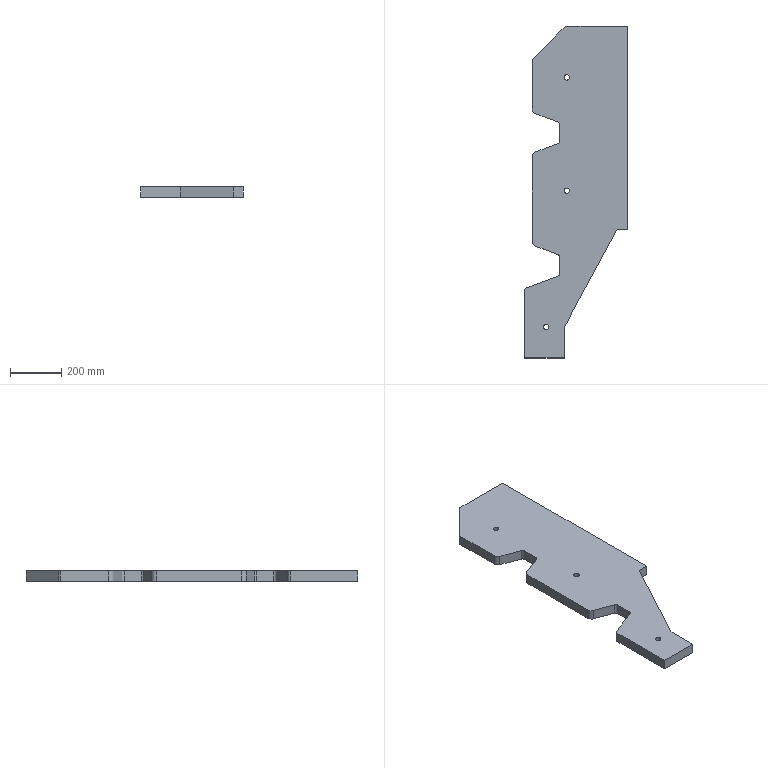Part | SolidWorks | features Fillet 3, ICE 2, 3DProfileFeature 1, Chamfer 1, Extrusion 1, HoleWzd 1 | 1 solid | 34 faces | box 399 x 1290 x 40 mm | volume 14647498 mm3 | plane 18 | cylinder 16 | commonest cylinder face diameters 20 x7 21 x6 40 x3
STEP:
#1=CARTESIAN_POINT('',(174.5,1090.,40.));
#2=VERTEX_POINT('',#1);
#3=CARTESIAN_POINT('',(153.5,1090.,40.));
#4=VERTEX_POINT('',#3);
#5=CARTESIAN_POINT('',(164.,1090.,40.));
#6=DIRECTION('',(0.,0.,-1.));
#7=DIRECTION('',(-1.,0.,0.));
#8=AXIS2_PLACEMENT_3D('',#5,#6,#7);
#9=CIRCLE('',#8,10.5);
#10=EDGE_CURVE('',#2,#4,#9,.T.);
#11=ORIENTED_EDGE('',*,*,#10,.F.);
#12=CARTESIAN_POINT('',(174.5,1090.,0.));
#13=VERTEX_POINT('',#12);
#14=CARTESIAN_POINT('',(174.5,1090.,0.));
#15=DIRECTION('',(0.,0.,-1.));
#16=VECTOR('',#15,1000.);
#17=LINE('',#14,#16);
#18=EDGE_CURVE('',#2,#13,#17,.T.);
#19=ORIENTED_EDGE('',*,*,#18,.T.);
#20=CARTESIAN_POINT('',(153.5,1090.,0.));
#21=VERTEX_POINT('',#20);
#22=CARTESIAN_POINT('',(164.,1090.,0.));
#23=DIRECTION('',(0.,0.,-1.));
#24=DIRECTION('',(-1.,0.,0.));
#25=AXIS2_PLACEMENT_3D('',#22,#23,#24);
#26=CIRCLE('',#25,10.5);
#27=EDGE_CURVE('',#13,#21,#26,.T.);
#28=ORIENTED_EDGE('',*,*,#27,.T.);
#29=CARTESIAN_POINT('',(153.5,1090.,0.));
#30=DIRECTION('',(0.,0.,-1.));
#31=VECTOR('',#30,1000.);
#32=LINE('',#29,#31);
#33=EDGE_CURVE('',#4,#21,#32,.T.);
#34=ORIENTED_EDGE('',*,*,#33,.F.);
#35=EDGE_LOOP('',(#11,#19,#28,#34));
#36=FACE_OUTER_BOUND('',#35,.T.);
#37=CARTESIAN_POINT('',(164.,1090.,0.));
#38=DIRECTION('',(0.,0.,-1.));
#39=DIRECTION('',(-1.,0.,0.));
#40=AXIS2_PLACEMENT_3D('',#37,#38,#39);
#41=CYLINDRICAL_SURFACE('',#40,10.5);
#42=ADVANCED_FACE('',(#36),#41,.F.);
#43=CARTESIAN_POINT('',(174.5,650.,40.));
#44=VERTEX_POINT('',#43);
#45=CARTESIAN_POINT('',(153.5,650.,40.));
#46=VERTEX_POINT('',#45);
#47=CARTESIAN_POINT('',(164.,650.,40.));
#48=DIRECTION('',(0.,0.,-1.));
#49=DIRECTION('',(-1.,0.,0.));
#50=AXIS2_PLACEMENT_3D('',#47,#48,#49);
#51=CIRCLE('',#50,10.5);
#52=EDGE_CURVE('',#44,#46,#51,.T.);
#53=ORIENTED_EDGE('',*,*,#52,.F.);
#54=CARTESIAN_POINT('',(174.5,650.,0.));
#55=VERTEX_POINT('',#54);
#56=CARTESIAN_POINT('',(174.5,650.,0.));
#57=DIRECTION('',(0.,0.,-1.));
#58=VECTOR('',#57,1000.);
#59=LINE('',#56,#58);
#60=EDGE_CURVE('',#44,#55,#59,.T.);
#61=ORIENTED_EDGE('',*,*,#60,.T.);
#62=CARTESIAN_POINT('',(153.5,650.,0.));
#63=VERTEX_POINT('',#62);
#64=CARTESIAN_POINT('',(164.,650.,0.));
#65=DIRECTION('',(0.,0.,-1.));
#66=DIRECTION('',(-1.,0.,0.));
#67=AXIS2_PLACEMENT_3D('',#64,#65,#66);
#68=CIRCLE('',#67,10.5);
#69=EDGE_CURVE('',#55,#63,#68,.T.);
#70=ORIENTED_EDGE('',*,*,#69,.T.);
#71=CARTESIAN_POINT('',(153.5,650.,0.));
#72=DIRECTION('',(0.,0.,-1.));
#73=VECTOR('',#72,1000.);
#74=LINE('',#71,#73);
#75=EDGE_CURVE('',#46,#63,#74,.T.);
#76=ORIENTED_EDGE('',*,*,#75,.F.);
#77=EDGE_LOOP('',(#53,#61,#70,#76));
#78=FACE_OUTER_BOUND('',#77,.T.);
#79=CARTESIAN_POINT('',(164.,650.,0.));
#80=DIRECTION('',(0.,0.,-1.));
#81=DIRECTION('',(-1.,0.,0.));
#82=AXIS2_PLACEMENT_3D('',#79,#80,#81);
#83=CYLINDRICAL_SURFACE('',#82,10.5);
#84=ADVANCED_FACE('',(#78),#83,.F.);
#85=CARTESIAN_POINT('',(94.5,120.,40.));
#86=VERTEX_POINT('',#85);
#87=CARTESIAN_POINT('',(73.5,120.,40.));
#88=VERTEX_POINT('',#87);
#89=CARTESIAN_POINT('',(84.,120.,40.));
#90=DIRECTION('',(0.,0.,-1.));
#91=DIRECTION('',(-1.,0.,0.));
#92=AXIS2_PLACEMENT_3D('',#89,#90,#91);
#93=CIRCLE('',#92,10.5);
#94=EDGE_CURVE('',#86,#88,#93,.T.);
#95=ORIENTED_EDGE('',*,*,#94,.F.);
#96=CARTESIAN_POINT('',(94.5,120.,0.));
#97=VERTEX_POINT('',#96);
#98=CARTESIAN_POINT('',(94.5,120.,0.));
#99=DIRECTION('',(0.,0.,-1.));
#100=VECTOR('',#99,1000.);
#101=LINE('',#98,#100);
#102=EDGE_CURVE('',#86,#97,#101,.T.);
#103=ORIENTED_EDGE('',*,*,#102,.T.);
#104=CARTESIAN_POINT('',(73.5,120.,0.));
#105=VERTEX_POINT('',#104);
#106=CARTESIAN_POINT('',(84.,120.,0.));
#107=DIRECTION('',(0.,0.,-1.));
#108=DIRECTION('',(-1.,0.,0.));
#109=AXIS2_PLACEMENT_3D('',#106,#107,#108);
#110=CIRCLE('',#109,10.5);
#111=EDGE_CURVE('',#97,#105,#110,.T.);
#112=ORIENTED_EDGE('',*,*,#111,.T.);
#113=CARTESIAN_POINT('',(73.5,120.,0.));
#114=DIRECTION('',(0.,0.,-1.));
#115=VECTOR('',#114,1000.);
#116=LINE('',#113,#115);
#117=EDGE_CURVE('',#88,#105,#116,.T.);
#118=ORIENTED_EDGE('',*,*,#117,.F.);
#119=EDGE_LOOP('',(#95,#103,#112,#118));
#120=FACE_OUTER_BOUND('',#119,.T.);
#121=CARTESIAN_POINT('',(84.,120.,0.));
#122=DIRECTION('',(0.,0.,-1.));
#123=DIRECTION('',(-1.,0.,0.));
#124=AXIS2_PLACEMENT_3D('',#121,#122,#123);
#125=CYLINDRICAL_SURFACE('',#124,10.5);
#126=ADVANCED_FACE('',(#120),#125,.F.);
#127=CARTESIAN_POINT('',(0.,263.04,40.));
#128=VERTEX_POINT('',#127);
#129=CARTESIAN_POINT('',(0.,0.,40.));
#130=VERTEX_POINT('',#129);
#131=CARTESIAN_POINT('',(0.,0.,40.));
#132=DIRECTION('',(0.,-1.,0.));
#133=VECTOR('',#132,1000.);
#134=LINE('',#131,#133);
#135=EDGE_CURVE('',#128,#130,#134,.T.);
#136=ORIENTED_EDGE('',*,*,#135,.F.);
#137=CARTESIAN_POINT('',(0.,263.04,0.));
#138=VERTEX_POINT('',#137);
#139=CARTESIAN_POINT('',(0.,263.04,40.));
#140=DIRECTION('',(0.,0.,-1.));
#141=VECTOR('',#140,1000.);
#142=LINE('',#139,#141);
#143=EDGE_CURVE('',#128,#138,#142,.T.);
#144=ORIENTED_EDGE('',*,*,#143,.T.);
#145=CARTESIAN_POINT('',(0.,0.,0.));
#146=VERTEX_POINT('',#145);
#147=CARTESIAN_POINT('',(0.,0.,0.));
#148=DIRECTION('',(0.,-1.,0.));
#149=VECTOR('',#148,1000.);
#150=LINE('',#147,#149);
#151=EDGE_CURVE('',#138,#146,#150,.T.);
#152=ORIENTED_EDGE('',*,*,#151,.T.);
#153=CARTESIAN_POINT('',(0.,0.,40.));
#154=DIRECTION('',(0.,0.,-1.));
#155=VECTOR('',#154,1000.);
#156=LINE('',#153,#155);
#157=EDGE_CURVE('',#130,#146,#156,.T.);
#158=ORIENTED_EDGE('',*,*,#157,.F.);
#159=EDGE_LOOP('',(#136,#144,#152,#158));
#160=FACE_OUTER_BOUND('',#159,.T.);
#161=CARTESIAN_POINT('',(0.,0.,40.));
#162=DIRECTION('',(1.,0.,0.));
#163=DIRECTION('',(0.,0.,-1.));
#164=AXIS2_PLACEMENT_3D('',#161,#162,#163);
#165=PLANE('',#164);
#166=ADVANCED_FACE('',(#160),#165,.F.);
#167=CARTESIAN_POINT('',(154.,0.,0.));
#168=VERTEX_POINT('',#167);
#169=CARTESIAN_POINT('',(0.,0.,0.));
#170=DIRECTION('',(1.,0.,0.));
#171=VECTOR('',#170,1000.);
#172=LINE('',#169,#171);
#173=EDGE_CURVE('',#146,#168,#172,.T.);
#174=ORIENTED_EDGE('',*,*,#173,.T.);
#175=CARTESIAN_POINT('',(154.,0.,40.));
#176=VERTEX_POINT('',#175);
#177=CARTESIAN_POINT('',(154.,0.,40.));
#178=DIRECTION('',(0.,0.,-1.));
#179=VECTOR('',#178,1000.);
#180=LINE('',#177,#179);
#181=EDGE_CURVE('',#176,#168,#180,.T.);
#182=ORIENTED_EDGE('',*,*,#181,.F.);
#183=CARTESIAN_POINT('',(0.,0.,40.));
#184=DIRECTION('',(1.,0.,0.));
#185=VECTOR('',#184,1000.);
#186=LINE('',#183,#185);
#187=EDGE_CURVE('',#130,#176,#186,.T.);
#188=ORIENTED_EDGE('',*,*,#187,.F.);
#189=ORIENTED_EDGE('',*,*,#157,.T.);
#190=EDGE_LOOP('',(#174,#182,#188,#189));
#191=FACE_OUTER_BOUND('',#190,.T.);
#192=CARTESIAN_POINT('',(0.,0.,40.));
#193=DIRECTION('',(0.,1.,0.));
#194=DIRECTION('',(0.,0.,1.));
#195=AXIS2_PLACEMENT_3D('',#192,#193,#194);
#196=PLANE('',#195);
#197=ADVANCED_FACE('',(#191),#196,.F.);
#198=CARTESIAN_POINT('',(154.,120.,0.));
#199=VERTEX_POINT('',#198);
#200=CARTESIAN_POINT('',(154.,0.,0.));
#201=DIRECTION('',(0.,1.,0.));
#202=VECTOR('',#201,1000.);
#203=LINE('',#200,#202);
#204=EDGE_CURVE('',#168,#199,#203,.T.);
#205=ORIENTED_EDGE('',*,*,#204,.T.);
#206=CARTESIAN_POINT('',(154.,120.,40.));
#207=VERTEX_POINT('',#206);
#208=CARTESIAN_POINT('',(154.,120.,40.));
#209=DIRECTION('',(0.,0.,-1.));
#210=VECTOR('',#209,1000.);
#211=LINE('',#208,#210);
#212=EDGE_CURVE('',#207,#199,#211,.T.);
#213=ORIENTED_EDGE('',*,*,#212,.F.);
#214=CARTESIAN_POINT('',(154.,0.,40.));
#215=DIRECTION('',(0.,1.,0.));
#216=VECTOR('',#215,1000.);
#217=LINE('',#214,#216);
#218=EDGE_CURVE('',#176,#207,#217,.T.);
#219=ORIENTED_EDGE('',*,*,#218,.F.);
#220=ORIENTED_EDGE('',*,*,#181,.T.);
#221=EDGE_LOOP('',(#205,#213,#219,#220));
#222=FACE_OUTER_BOUND('',#221,.T.);
#223=CARTESIAN_POINT('',(154.,0.,40.));
#224=DIRECTION('',(-1.,0.,0.));
#225=DIRECTION('',(0.,0.,1.));
#226=AXIS2_PLACEMENT_3D('',#223,#224,#225);
#227=PLANE('',#226);
#228=ADVANCED_FACE('',(#222),#227,.F.);
#229=CARTESIAN_POINT('',(359.,500.,0.));
#230=VERTEX_POINT('',#229);
#231=CARTESIAN_POINT('',(154.,120.,0.));
#232=DIRECTION('',(0.4748,0.8801,0.));
#233=VECTOR('',#232,1000.);
#234=LINE('',#231,#233);
#235=EDGE_CURVE('',#199,#230,#234,.T.);
#236=ORIENTED_EDGE('',*,*,#235,.T.);
#237=CARTESIAN_POINT('',(359.,500.,40.));
#238=VERTEX_POINT('',#237);
#239=CARTESIAN_POINT('',(359.,500.,40.));
#240=DIRECTION('',(0.,0.,-1.));
#241=VECTOR('',#240,1000.);
#242=LINE('',#239,#241);
#243=EDGE_CURVE('',#238,#230,#242,.T.);
#244=ORIENTED_EDGE('',*,*,#243,.F.);
#245=CARTESIAN_POINT('',(154.,120.,40.));
#246=DIRECTION('',(0.4748,0.8801,0.));
#247=VECTOR('',#246,1000.);
#248=LINE('',#245,#247);
#249=EDGE_CURVE('',#207,#238,#248,.T.);
#250=ORIENTED_EDGE('',*,*,#249,.F.);
#251=ORIENTED_EDGE('',*,*,#212,.T.);
#252=EDGE_LOOP('',(#236,#244,#250,#251));
#253=FACE_OUTER_BOUND('',#252,.T.);
#254=CARTESIAN_POINT('',(154.,120.,40.));
#255=DIRECTION('',(-0.8801,0.4748,0.));
#256=DIRECTION('',(-0.4748,-0.8801,0.));
#257=AXIS2_PLACEMENT_3D('',#254,#255,#256);
#258=PLANE('',#257);
#259=ADVANCED_FACE('',(#253),#258,.F.);
#260=CARTESIAN_POINT('',(399.,500.,0.));
#261=VERTEX_POINT('',#260);
#262=CARTESIAN_POINT('',(359.,500.,0.));
#263=DIRECTION('',(1.,0.,0.));
#264=VECTOR('',#263,1000.);
#265=LINE('',#262,#264);
#266=EDGE_CURVE('',#230,#261,#265,.T.);
#267=ORIENTED_EDGE('',*,*,#266,.T.);
#268=CARTESIAN_POINT('',(399.,500.,40.));
#269=VERTEX_POINT('',#268);
#270=CARTESIAN_POINT('',(399.,500.,40.));
#271=DIRECTION('',(0.,0.,-1.));
#272=VECTOR('',#271,1000.);
#273=LINE('',#270,#272);
#274=EDGE_CURVE('',#269,#261,#273,.T.);
#275=ORIENTED_EDGE('',*,*,#274,.F.);
#276=CARTESIAN_POINT('',(359.,500.,40.));
#277=DIRECTION('',(1.,0.,0.));
#278=VECTOR('',#277,1000.);
#279=LINE('',#276,#278);
#280=EDGE_CURVE('',#238,#269,#279,.T.);
#281=ORIENTED_EDGE('',*,*,#280,.F.);
#282=ORIENTED_EDGE('',*,*,#243,.T.);
#283=EDGE_LOOP('',(#267,#275,#281,#282));
#284=FACE_OUTER_BOUND('',#283,.T.);
#285=CARTESIAN_POINT('',(359.,500.,40.));
#286=DIRECTION('',(0.,1.,0.));
#287=DIRECTION('',(0.,0.,1.));
#288=AXIS2_PLACEMENT_3D('',#285,#286,#287);
#289=PLANE('',#288);
#290=ADVANCED_FACE('',(#284),#289,.F.);
#291=CARTESIAN_POINT('',(399.,1290.,0.));
#292=VERTEX_POINT('',#291);
#293=CARTESIAN_POINT('',(399.,500.,0.));
#294=DIRECTION('',(0.,1.,0.));
#295=VECTOR('',#294,1000.);
#296=LINE('',#293,#295);
#297=EDGE_CURVE('',#261,#292,#296,.T.);
#298=ORIENTED_EDGE('',*,*,#297,.T.);
#299=CARTESIAN_POINT('',(399.,1290.,40.));
#300=VERTEX_POINT('',#299);
#301=CARTESIAN_POINT('',(399.,1290.,40.));
#302=DIRECTION('',(0.,0.,-1.));
#303=VECTOR('',#302,1000.);
#304=LINE('',#301,#303);
#305=EDGE_CURVE('',#300,#292,#304,.T.);
#306=ORIENTED_EDGE('',*,*,#305,.F.);
#307=CARTESIAN_POINT('',(399.,500.,40.));
#308=DIRECTION('',(0.,1.,0.));
#309=VECTOR('',#308,1000.);
#310=LINE('',#307,#309);
#311=EDGE_CURVE('',#269,#300,#310,.T.);
#312=ORIENTED_EDGE('',*,*,#311,.F.);
#313=ORIENTED_EDGE('',*,*,#274,.T.);
#314=EDGE_LOOP('',(#298,#306,#312,#313));
#315=FACE_OUTER_BOUND('',#314,.T.);
#316=CARTESIAN_POINT('',(399.,500.,40.));
#317=DIRECTION('',(-1.,0.,0.));
#318=DIRECTION('',(0.,0.,1.));
#319=AXIS2_PLACEMENT_3D('',#316,#317,#318);
#320=PLANE('',#319);
#321=ADVANCED_FACE('',(#315),#320,.F.);
#322=CARTESIAN_POINT('',(164.142,1290.,0.));
#323=VERTEX_POINT('',#322);
#324=CARTESIAN_POINT('',(0.,1290.,0.));
#325=DIRECTION('',(-1.,0.,0.));
#326=VECTOR('',#325,1000.);
#327=LINE('',#324,#326);
#328=EDGE_CURVE('',#292,#323,#327,.T.);
#329=ORIENTED_EDGE('',*,*,#328,.T.);
#330=CARTESIAN_POINT('',(164.142,1290.,40.));
#331=VERTEX_POINT('',#330);
#332=CARTESIAN_POINT('',(164.142,1290.,40.));
#333=DIRECTION('',(0.,0.,1.));
#334=VECTOR('',#333,1000.);
#335=LINE('',#332,#334);
#336=EDGE_CURVE('',#323,#331,#335,.T.);
#337=ORIENTED_EDGE('',*,*,#336,.T.);
#338=CARTESIAN_POINT('',(0.,1290.,40.));
#339=DIRECTION('',(-1.,0.,0.));
#340=VECTOR('',#339,1000.);
#341=LINE('',#338,#340);
#342=EDGE_CURVE('',#300,#331,#341,.T.);
#343=ORIENTED_EDGE('',*,*,#342,.F.);
#344=ORIENTED_EDGE('',*,*,#305,.T.);
#345=EDGE_LOOP('',(#329,#337,#343,#344));
#346=FACE_OUTER_BOUND('',#345,.T.);
#347=CARTESIAN_POINT('',(0.,1290.,40.));
#348=DIRECTION('',(0.,-1.,0.));
#349=DIRECTION('',(0.,0.,-1.));
#350=AXIS2_PLACEMENT_3D('',#347,#348,#349);
#351=PLANE('',#350);
#352=ADVANCED_FACE('',(#346),#351,.F.);
#353=ORIENTED_EDGE('',*,*,#342,.T.);
#354=CARTESIAN_POINT('',(157.071,1287.071,40.));
#355=VERTEX_POINT('',#354);
#356=CARTESIAN_POINT('',(164.142,1280.,40.));
#357=DIRECTION('',(0.,0.,1.));
#358=DIRECTION('',(-1.,0.,0.));
#359=AXIS2_PLACEMENT_3D('',#356,#357,#358);
#360=CIRCLE('',#359,10.);
#361=EDGE_CURVE('',#331,#355,#360,.T.);
#362=ORIENTED_EDGE('',*,*,#361,.T.);
#363=CARTESIAN_POINT('',(32.929,1162.929,40.));
#364=VERTEX_POINT('',#363);
#365=CARTESIAN_POINT('',(0.,1130.,40.));
#366=DIRECTION('',(-0.7071,-0.7071,0.));
#367=VECTOR('',#366,1000.);
#368=LINE('',#365,#367);
#369=EDGE_CURVE('',#355,#364,#368,.T.);
#370=ORIENTED_EDGE('',*,*,#369,.T.);
#371=CARTESIAN_POINT('',(30.,1155.858,40.));
#372=VERTEX_POINT('',#371);
#373=CARTESIAN_POINT('',(40.,1155.858,40.));
#374=DIRECTION('',(0.,0.,1.));
#375=DIRECTION('',(-1.,0.,0.));
#376=AXIS2_PLACEMENT_3D('',#373,#374,#375);
#377=CIRCLE('',#376,10.);
#378=EDGE_CURVE('',#364,#372,#377,.T.);
#379=ORIENTED_EDGE('',*,*,#378,.T.);
#380=CARTESIAN_POINT('',(30.,967.809,40.));
#381=VERTEX_POINT('',#380);
#382=CARTESIAN_POINT('',(30.,337.181,40.));
#383=DIRECTION('',(0.,-1.,0.));
#384=VECTOR('',#383,1000.);
#385=LINE('',#382,#384);
#386=EDGE_CURVE('',#372,#381,#385,.T.);
#387=ORIENTED_EDGE('',*,*,#386,.T.);
#388=CARTESIAN_POINT('',(43.054,949.054,40.));
#389=VERTEX_POINT('',#388);
#390=CARTESIAN_POINT('',(50.,967.809,40.));
#391=DIRECTION('',(0.,0.,1.));
#392=DIRECTION('',(-1.,0.,0.));
#393=AXIS2_PLACEMENT_3D('',#390,#391,#392);
#394=CIRCLE('',#393,20.);
#395=EDGE_CURVE('',#381,#389,#394,.T.);
#396=ORIENTED_EDGE('',*,*,#395,.T.);
#397=CARTESIAN_POINT('',(128.473,917.417,40.));
#398=VERTEX_POINT('',#397);
#399=CARTESIAN_POINT('',(0.,965.,40.));
#400=DIRECTION('',(0.9377,-0.3473,0.));
#401=VECTOR('',#400,1000.);
#402=LINE('',#399,#401);
#403=EDGE_CURVE('',#389,#398,#402,.T.);
#404=ORIENTED_EDGE('',*,*,#403,.T.);
#405=CARTESIAN_POINT('',(135.,908.04,40.));
#406=VERTEX_POINT('',#405);
#407=CARTESIAN_POINT('',(125.,908.04,40.));
#408=DIRECTION('',(0.,0.,-1.));
#409=DIRECTION('',(-1.,0.,0.));
#410=AXIS2_PLACEMENT_3D('',#407,#408,#409);
#411=CIRCLE('',#410,10.);
#412=EDGE_CURVE('',#398,#406,#411,.T.);
#413=ORIENTED_EDGE('',*,*,#412,.T.);
#414=CARTESIAN_POINT('',(135.,841.96,40.));
#415=VERTEX_POINT('',#414);
#416=CARTESIAN_POINT('',(135.,835.,40.));
#417=DIRECTION('',(0.,-1.,0.));
#418=VECTOR('',#417,1000.);
#419=LINE('',#416,#418);
#420=EDGE_CURVE('',#406,#415,#419,.T.);
#421=ORIENTED_EDGE('',*,*,#420,.T.);
#422=CARTESIAN_POINT('',(128.473,832.583,40.));
#423=VERTEX_POINT('',#422);
#424=CARTESIAN_POINT('',(125.,841.96,40.));
#425=DIRECTION('',(0.,0.,-1.));
#426=DIRECTION('',(-1.,0.,0.));
#427=AXIS2_PLACEMENT_3D('',#424,#425,#426);
#428=CIRCLE('',#427,10.);
#429=EDGE_CURVE('',#415,#423,#428,.T.);
#430=ORIENTED_EDGE('',*,*,#429,.T.);
#431=CARTESIAN_POINT('',(43.054,800.946,40.));
#432=VERTEX_POINT('',#431);
#433=CARTESIAN_POINT('',(135.,835.,40.));
#434=DIRECTION('',(-0.9377,-0.3473,0.));
#435=VECTOR('',#434,1000.);
#436=LINE('',#433,#435);
#437=EDGE_CURVE('',#423,#432,#436,.T.);
#438=ORIENTED_EDGE('',*,*,#437,.T.);
#439=CARTESIAN_POINT('',(30.,782.191,40.));
#440=VERTEX_POINT('',#439);
#441=CARTESIAN_POINT('',(50.,782.191,40.));
#442=DIRECTION('',(0.,0.,1.));
#443=DIRECTION('',(-1.,0.,0.));
#444=AXIS2_PLACEMENT_3D('',#441,#442,#443);
#445=CIRCLE('',#444,20.);
#446=EDGE_CURVE('',#432,#440,#445,.T.);
#447=ORIENTED_EDGE('',*,*,#446,.T.);
#448=CARTESIAN_POINT('',(30.,452.809,40.));
#449=VERTEX_POINT('',#448);
#450=CARTESIAN_POINT('',(30.,337.181,40.));
#451=DIRECTION('',(0.,-1.,0.));
#452=VECTOR('',#451,1000.);
#453=LINE('',#450,#452);
#454=EDGE_CURVE('',#440,#449,#453,.T.);
#455=ORIENTED_EDGE('',*,*,#454,.T.);
#456=CARTESIAN_POINT('',(43.054,434.054,40.));
#457=VERTEX_POINT('',#456);
#458=CARTESIAN_POINT('',(50.,452.809,40.));
#459=DIRECTION('',(0.,0.,1.));
#460=DIRECTION('',(-1.,0.,0.));
#461=AXIS2_PLACEMENT_3D('',#458,#459,#460);
#462=CIRCLE('',#461,20.);
#463=EDGE_CURVE('',#449,#457,#462,.T.);
#464=ORIENTED_EDGE('',*,*,#463,.T.);
#465=CARTESIAN_POINT('',(128.473,402.417,40.));
#466=VERTEX_POINT('',#465);
#467=CARTESIAN_POINT('',(135.,400.,40.));
#468=DIRECTION('',(0.9377,-0.3473,0.));
#469=VECTOR('',#468,1000.);
#470=LINE('',#467,#469);
#471=EDGE_CURVE('',#457,#466,#470,.T.);
#472=ORIENTED_EDGE('',*,*,#471,.T.);
#473=CARTESIAN_POINT('',(135.,393.04,40.));
#474=VERTEX_POINT('',#473);
#475=CARTESIAN_POINT('',(125.,393.04,40.));
#476=DIRECTION('',(0.,0.,-1.));
#477=DIRECTION('',(-1.,0.,0.));
#478=AXIS2_PLACEMENT_3D('',#475,#476,#477);
#479=CIRCLE('',#478,10.);
#480=EDGE_CURVE('',#466,#474,#479,.T.);
#481=ORIENTED_EDGE('',*,*,#480,.T.);
#482=CARTESIAN_POINT('',(135.,326.96,40.));
#483=VERTEX_POINT('',#482);
#484=CARTESIAN_POINT('',(135.,400.,40.));
#485=DIRECTION('',(0.,-1.,0.));
#486=VECTOR('',#485,1000.);
#487=LINE('',#484,#486);
#488=EDGE_CURVE('',#474,#483,#487,.T.);
#489=ORIENTED_EDGE('',*,*,#488,.T.);
#490=CARTESIAN_POINT('',(128.473,317.583,40.));
#491=VERTEX_POINT('',#490);
#492=CARTESIAN_POINT('',(125.,326.96,40.));
#493=DIRECTION('',(0.,0.,-1.));
#494=DIRECTION('',(-1.,0.,0.));
#495=AXIS2_PLACEMENT_3D('',#492,#493,#494);
#496=CIRCLE('',#495,10.);
#497=EDGE_CURVE('',#483,#491,#496,.T.);
#498=ORIENTED_EDGE('',*,*,#497,.T.);
#499=CARTESIAN_POINT('',(6.527,272.417,40.));
#500=VERTEX_POINT('',#499);
#501=CARTESIAN_POINT('',(0.,270.,40.));
#502=DIRECTION('',(-0.9377,-0.3473,0.));
#503=VECTOR('',#502,1000.);
#504=LINE('',#501,#503);
#505=EDGE_CURVE('',#491,#500,#504,.T.);
#506=ORIENTED_EDGE('',*,*,#505,.T.);
#507=CARTESIAN_POINT('',(10.,263.04,40.));
#508=DIRECTION('',(0.,0.,1.));
#509=DIRECTION('',(-1.,0.,0.));
#510=AXIS2_PLACEMENT_3D('',#507,#508,#509);
#511=CIRCLE('',#510,10.);
#512=EDGE_CURVE('',#500,#128,#511,.T.);
#513=ORIENTED_EDGE('',*,*,#512,.T.);
#514=ORIENTED_EDGE('',*,*,#135,.T.);
#515=ORIENTED_EDGE('',*,*,#187,.T.);
#516=ORIENTED_EDGE('',*,*,#218,.T.);
#517=ORIENTED_EDGE('',*,*,#249,.T.);
#518=ORIENTED_EDGE('',*,*,#280,.T.);
#519=ORIENTED_EDGE('',*,*,#311,.T.);
#520=EDGE_LOOP('',(#353,#362,#370,#379,#387,#396,#404,#413,#421,#430,#438,#447,#455,#464,#472,#481,#489,#498,#506,#513,#514,#515,#516,#517,#518,#519));
#521=FACE_OUTER_BOUND('',#520,.T.);
#522=CARTESIAN_POINT('',(164.,1090.,40.));
#523=DIRECTION('',(0.,0.,-1.));
#524=DIRECTION('',(-1.,0.,0.));
#525=AXIS2_PLACEMENT_3D('',#522,#523,#524);
#526=CIRCLE('',#525,10.5);
#527=EDGE_CURVE('',#4,#2,#526,.T.);
#528=ORIENTED_EDGE('',*,*,#527,.T.);
#529=ORIENTED_EDGE('',*,*,#10,.T.);
#530=EDGE_LOOP('',(#528,#529));
#531=FACE_BOUND('',#530,.T.);
#532=CARTESIAN_POINT('',(164.,650.,40.));
#533=DIRECTION('',(0.,0.,-1.));
#534=DIRECTION('',(-1.,0.,0.));
#535=AXIS2_PLACEMENT_3D('',#532,#533,#534);
#536=CIRCLE('',#535,10.5);
#537=EDGE_CURVE('',#46,#44,#536,.T.);
#538=ORIENTED_EDGE('',*,*,#537,.T.);
#539=ORIENTED_EDGE('',*,*,#52,.T.);
#540=EDGE_LOOP('',(#538,#539));
#541=FACE_BOUND('',#540,.T.);
#542=CARTESIAN_POINT('',(84.,120.,40.));
#543=DIRECTION('',(0.,0.,-1.));
#544=DIRECTION('',(-1.,0.,0.));
#545=AXIS2_PLACEMENT_3D('',#542,#543,#544);
#546=CIRCLE('',#545,10.5);
#547=EDGE_CURVE('',#88,#86,#546,.T.);
#548=ORIENTED_EDGE('',*,*,#547,.T.);
#549=ORIENTED_EDGE('',*,*,#94,.T.);
#550=EDGE_LOOP('',(#548,#549));
#551=FACE_BOUND('',#550,.T.);
#552=CARTESIAN_POINT('',(0.,0.,40.));
#553=DIRECTION('',(0.,0.,-1.));
#554=DIRECTION('',(-1.,0.,0.));
#555=AXIS2_PLACEMENT_3D('',#552,#553,#554);
#556=PLANE('',#555);
#557=ADVANCED_FACE('',(#521,#531,#541,#551),#556,.F.);
#558=CARTESIAN_POINT('',(32.929,1162.929,0.));
#559=VERTEX_POINT('',#558);
#560=CARTESIAN_POINT('',(157.071,1287.071,0.));
#561=VERTEX_POINT('',#560);
#562=CARTESIAN_POINT('',(-565.,565.,0.));
#563=DIRECTION('',(0.7071,0.7071,0.));
#564=VECTOR('',#563,1000.);
#565=LINE('',#562,#564);
#566=EDGE_CURVE('',#559,#561,#565,.T.);
#567=ORIENTED_EDGE('',*,*,#566,.T.);
#568=CARTESIAN_POINT('',(164.142,1280.,0.));
#569=DIRECTION('',(0.,0.,-1.));
#570=DIRECTION('',(-1.,0.,0.));
#571=AXIS2_PLACEMENT_3D('',#568,#569,#570);
#572=CIRCLE('',#571,10.);
#573=EDGE_CURVE('',#561,#323,#572,.T.);
#574=ORIENTED_EDGE('',*,*,#573,.T.);
#575=ORIENTED_EDGE('',*,*,#328,.F.);
#576=ORIENTED_EDGE('',*,*,#297,.F.);
#577=ORIENTED_EDGE('',*,*,#266,.F.);
#578=ORIENTED_EDGE('',*,*,#235,.F.);
#579=ORIENTED_EDGE('',*,*,#204,.F.);
#580=ORIENTED_EDGE('',*,*,#173,.F.);
#581=ORIENTED_EDGE('',*,*,#151,.F.);
#582=CARTESIAN_POINT('',(6.527,272.417,0.));
#583=VERTEX_POINT('',#582);
#584=CARTESIAN_POINT('',(10.,263.04,0.));
#585=DIRECTION('',(0.,0.,-1.));
#586=DIRECTION('',(-1.,0.,0.));
#587=AXIS2_PLACEMENT_3D('',#584,#585,#586);
#588=CIRCLE('',#587,10.);
#589=EDGE_CURVE('',#138,#583,#588,.T.);
#590=ORIENTED_EDGE('',*,*,#589,.T.);
#591=CARTESIAN_POINT('',(128.473,317.583,0.));
#592=VERTEX_POINT('',#591);
#593=CARTESIAN_POINT('',(0.,270.,0.));
#594=DIRECTION('',(-0.9377,-0.3473,0.));
#595=VECTOR('',#594,1000.);
#596=LINE('',#593,#595);
#597=EDGE_CURVE('',#592,#583,#596,.T.);
#598=ORIENTED_EDGE('',*,*,#597,.F.);
#599=CARTESIAN_POINT('',(135.,326.96,0.));
#600=VERTEX_POINT('',#599);
#601=CARTESIAN_POINT('',(125.,326.96,0.));
#602=DIRECTION('',(0.,0.,1.));
#603=DIRECTION('',(-1.,0.,0.));
#604=AXIS2_PLACEMENT_3D('',#601,#602,#603);
#605=CIRCLE('',#604,10.);
#606=EDGE_CURVE('',#592,#600,#605,.T.);
#607=ORIENTED_EDGE('',*,*,#606,.T.);
#608=CARTESIAN_POINT('',(135.,393.04,0.));
#609=VERTEX_POINT('',#608);
#610=CARTESIAN_POINT('',(135.,400.,0.));
#611=DIRECTION('',(0.,-1.,0.));
#612=VECTOR('',#611,1000.);
#613=LINE('',#610,#612);
#614=EDGE_CURVE('',#609,#600,#613,.T.);
#615=ORIENTED_EDGE('',*,*,#614,.F.);
#616=CARTESIAN_POINT('',(128.473,402.417,0.));
#617=VERTEX_POINT('',#616);
#618=CARTESIAN_POINT('',(125.,393.04,0.));
#619=DIRECTION('',(0.,0.,1.));
#620=DIRECTION('',(-1.,0.,0.));
#621=AXIS2_PLACEMENT_3D('',#618,#619,#620);
#622=CIRCLE('',#621,10.);
#623=EDGE_CURVE('',#609,#617,#622,.T.);
#624=ORIENTED_EDGE('',*,*,#623,.T.);
#625=CARTESIAN_POINT('',(43.054,434.054,0.));
#626=VERTEX_POINT('',#625);
#627=CARTESIAN_POINT('',(135.,400.,0.));
#628=DIRECTION('',(0.9377,-0.3473,0.));
#629=VECTOR('',#628,1000.);
#630=LINE('',#627,#629);
#631=EDGE_CURVE('',#626,#617,#630,.T.);
#632=ORIENTED_EDGE('',*,*,#631,.F.);
#633=CARTESIAN_POINT('',(30.,452.809,0.));
#634=VERTEX_POINT('',#633);
#635=CARTESIAN_POINT('',(50.,452.809,0.));
#636=DIRECTION('',(0.,0.,-1.));
#637=DIRECTION('',(-1.,0.,0.));
#638=AXIS2_PLACEMENT_3D('',#635,#636,#637);
#639=CIRCLE('',#638,20.);
#640=EDGE_CURVE('',#626,#634,#639,.T.);
#641=ORIENTED_EDGE('',*,*,#640,.T.);
#642=CARTESIAN_POINT('',(30.,782.191,0.));
#643=VERTEX_POINT('',#642);
#644=CARTESIAN_POINT('',(30.,337.181,0.));
#645=DIRECTION('',(0.,-1.,0.));
#646=VECTOR('',#645,1000.);
#647=LINE('',#644,#646);
#648=EDGE_CURVE('',#643,#634,#647,.T.);
#649=ORIENTED_EDGE('',*,*,#648,.F.);
#650=CARTESIAN_POINT('',(43.054,800.946,0.));
#651=VERTEX_POINT('',#650);
#652=CARTESIAN_POINT('',(50.,782.191,0.));
#653=DIRECTION('',(0.,0.,-1.));
#654=DIRECTION('',(-1.,0.,0.));
#655=AXIS2_PLACEMENT_3D('',#652,#653,#654);
#656=CIRCLE('',#655,20.);
#657=EDGE_CURVE('',#643,#651,#656,.T.);
#658=ORIENTED_EDGE('',*,*,#657,.T.);
#659=CARTESIAN_POINT('',(128.473,832.583,0.));
#660=VERTEX_POINT('',#659);
#661=CARTESIAN_POINT('',(135.,835.,0.));
#662=DIRECTION('',(-0.9377,-0.3473,0.));
#663=VECTOR('',#662,1000.);
#664=LINE('',#661,#663);
#665=EDGE_CURVE('',#660,#651,#664,.T.);
#666=ORIENTED_EDGE('',*,*,#665,.F.);
#667=CARTESIAN_POINT('',(135.,841.96,0.));
#668=VERTEX_POINT('',#667);
#669=CARTESIAN_POINT('',(125.,841.96,0.));
#670=DIRECTION('',(0.,0.,1.));
#671=DIRECTION('',(-1.,0.,0.));
#672=AXIS2_PLACEMENT_3D('',#669,#670,#671);
#673=CIRCLE('',#672,10.);
#674=EDGE_CURVE('',#660,#668,#673,.T.);
#675=ORIENTED_EDGE('',*,*,#674,.T.);
#676=CARTESIAN_POINT('',(135.,908.04,0.));
#677=VERTEX_POINT('',#676);
#678=CARTESIAN_POINT('',(135.,835.,0.));
#679=DIRECTION('',(0.,-1.,0.));
#680=VECTOR('',#679,1000.);
#681=LINE('',#678,#680);
#682=EDGE_CURVE('',#677,#668,#681,.T.);
#683=ORIENTED_EDGE('',*,*,#682,.F.);
#684=CARTESIAN_POINT('',(128.473,917.417,0.));
#685=VERTEX_POINT('',#684);
#686=CARTESIAN_POINT('',(125.,908.04,0.));
#687=DIRECTION('',(0.,0.,1.));
#688=DIRECTION('',(-1.,0.,0.));
#689=AXIS2_PLACEMENT_3D('',#686,#687,#688);
#690=CIRCLE('',#689,10.);
#691=EDGE_CURVE('',#677,#685,#690,.T.);
#692=ORIENTED_EDGE('',*,*,#691,.T.);
#693=CARTESIAN_POINT('',(43.054,949.054,0.));
#694=VERTEX_POINT('',#693);
#695=CARTESIAN_POINT('',(0.,965.,0.));
#696=DIRECTION('',(0.9377,-0.3473,0.));
#697=VECTOR('',#696,1000.);
#698=LINE('',#695,#697);
#699=EDGE_CURVE('',#694,#685,#698,.T.);
#700=ORIENTED_EDGE('',*,*,#699,.F.);
#701=CARTESIAN_POINT('',(30.,967.809,0.));
#702=VERTEX_POINT('',#701);
#703=CARTESIAN_POINT('',(50.,967.809,0.));
#704=DIRECTION('',(0.,0.,-1.));
#705=DIRECTION('',(-1.,0.,0.));
#706=AXIS2_PLACEMENT_3D('',#703,#704,#705);
#707=CIRCLE('',#706,20.);
#708=EDGE_CURVE('',#694,#702,#707,.T.);
#709=ORIENTED_EDGE('',*,*,#708,.T.);
#710=CARTESIAN_POINT('',(30.,1155.858,0.));
#711=VERTEX_POINT('',#710);
#712=CARTESIAN_POINT('',(30.,337.181,0.));
#713=DIRECTION('',(0.,-1.,0.));
#714=VECTOR('',#713,1000.);
#715=LINE('',#712,#714);
#716=EDGE_CURVE('',#711,#702,#715,.T.);
#717=ORIENTED_EDGE('',*,*,#716,.F.);
#718=CARTESIAN_POINT('',(40.,1155.858,0.));
#719=DIRECTION('',(0.,0.,-1.));
#720=DIRECTION('',(-1.,0.,0.));
#721=AXIS2_PLACEMENT_3D('',#718,#719,#720);
#722=CIRCLE('',#721,10.);
#723=EDGE_CURVE('',#711,#559,#722,.T.);
#724=ORIENTED_EDGE('',*,*,#723,.T.);
#725=EDGE_LOOP('',(#567,#574,#575,#576,#577,#578,#579,#580,#581,#590,#598,#607,#615,#624,#632,#641,#649,#658,#666,#675,#683,#692,#700,#709,#717,#724));
#726=FACE_OUTER_BOUND('',#725,.T.);
#727=CARTESIAN_POINT('',(164.,1090.,0.));
#728=DIRECTION('',(0.,0.,-1.));
#729=DIRECTION('',(-1.,0.,0.));
#730=AXIS2_PLACEMENT_3D('',#727,#728,#729);
#731=CIRCLE('',#730,10.5);
#732=EDGE_CURVE('',#21,#13,#731,.T.);
#733=ORIENTED_EDGE('',*,*,#732,.F.);
#734=ORIENTED_EDGE('',*,*,#27,.F.);
#735=EDGE_LOOP('',(#733,#734));
#736=FACE_BOUND('',#735,.T.);
#737=CARTESIAN_POINT('',(164.,650.,0.));
#738=DIRECTION('',(0.,0.,-1.));
#739=DIRECTION('',(-1.,0.,0.));
#740=AXIS2_PLACEMENT_3D('',#737,#738,#739);
#741=CIRCLE('',#740,10.5);
#742=EDGE_CURVE('',#63,#55,#741,.T.);
#743=ORIENTED_EDGE('',*,*,#742,.F.);
#744=ORIENTED_EDGE('',*,*,#69,.F.);
#745=EDGE_LOOP('',(#743,#744));
#746=FACE_BOUND('',#745,.T.);
#747=CARTESIAN_POINT('',(84.,120.,0.));
#748=DIRECTION('',(0.,0.,-1.));
#749=DIRECTION('',(-1.,0.,0.));
#750=AXIS2_PLACEMENT_3D('',#747,#748,#749);
#751=CIRCLE('',#750,10.5);
#752=EDGE_CURVE('',#105,#97,#751,.T.);
#753=ORIENTED_EDGE('',*,*,#752,.F.);
#754=ORIENTED_EDGE('',*,*,#111,.F.);
#755=EDGE_LOOP('',(#753,#754));
#756=FACE_BOUND('',#755,.T.);
#757=CARTESIAN_POINT('',(0.,0.,0.));
#758=DIRECTION('',(0.,0.,-1.));
#759=DIRECTION('',(-1.,0.,0.));
#760=AXIS2_PLACEMENT_3D('',#757,#758,#759);
#761=PLANE('',#760);
#762=ADVANCED_FACE('',(#726,#736,#746,#756),#761,.T.);
#763=ORIENTED_EDGE('',*,*,#369,.F.);
#764=CARTESIAN_POINT('',(157.071,1287.071,0.));
#765=DIRECTION('',(0.,0.,-1.));
#766=VECTOR('',#765,1000.);
#767=LINE('',#764,#766);
#768=EDGE_CURVE('',#355,#561,#767,.T.);
#769=ORIENTED_EDGE('',*,*,#768,.T.);
#770=ORIENTED_EDGE('',*,*,#566,.F.);
#771=CARTESIAN_POINT('',(32.929,1162.929,40.));
#772=DIRECTION('',(0.,0.,1.));
#773=VECTOR('',#772,1000.);
#774=LINE('',#771,#773);
#775=EDGE_CURVE('',#559,#364,#774,.T.);
#776=ORIENTED_EDGE('',*,*,#775,.T.);
#777=EDGE_LOOP('',(#763,#769,#770,#776));
#778=FACE_OUTER_BOUND('',#777,.T.);
#779=CARTESIAN_POINT('',(0.,1130.,40.));
#780=DIRECTION('',(0.7071,-0.7071,0.));
#781=DIRECTION('',(0.,0.,-1.));
#782=AXIS2_PLACEMENT_3D('',#779,#780,#781);
#783=PLANE('',#782);
#784=ADVANCED_FACE('',(#778),#783,.F.);
#785=ORIENTED_EDGE('',*,*,#102,.F.);
#786=ORIENTED_EDGE('',*,*,#547,.F.);
#787=ORIENTED_EDGE('',*,*,#117,.T.);
#788=ORIENTED_EDGE('',*,*,#752,.T.);
#789=EDGE_LOOP('',(#785,#786,#787,#788));
#790=FACE_OUTER_BOUND('',#789,.T.);
#791=CARTESIAN_POINT('',(84.,120.,0.));
#792=DIRECTION('',(0.,0.,-1.));
#793=DIRECTION('',(-1.,0.,0.));
#794=AXIS2_PLACEMENT_3D('',#791,#792,#793);
#795=CYLINDRICAL_SURFACE('',#794,10.5);
#796=ADVANCED_FACE('',(#790),#795,.F.);
#797=ORIENTED_EDGE('',*,*,#60,.F.);
#798=ORIENTED_EDGE('',*,*,#537,.F.);
#799=ORIENTED_EDGE('',*,*,#75,.T.);
#800=ORIENTED_EDGE('',*,*,#742,.T.);
#801=EDGE_LOOP('',(#797,#798,#799,#800));
#802=FACE_OUTER_BOUND('',#801,.T.);
#803=CARTESIAN_POINT('',(164.,650.,0.));
#804=DIRECTION('',(0.,0.,-1.));
#805=DIRECTION('',(-1.,0.,0.));
#806=AXIS2_PLACEMENT_3D('',#803,#804,#805);
#807=CYLINDRICAL_SURFACE('',#806,10.5);
#808=ADVANCED_FACE('',(#802),#807,.F.);
#809=ORIENTED_EDGE('',*,*,#18,.F.);
#810=ORIENTED_EDGE('',*,*,#527,.F.);
#811=ORIENTED_EDGE('',*,*,#33,.T.);
#812=ORIENTED_EDGE('',*,*,#732,.T.);
#813=EDGE_LOOP('',(#809,#810,#811,#812));
#814=FACE_OUTER_BOUND('',#813,.T.);
#815=CARTESIAN_POINT('',(164.,1090.,0.));
#816=DIRECTION('',(0.,0.,-1.));
#817=DIRECTION('',(-1.,0.,0.));
#818=AXIS2_PLACEMENT_3D('',#815,#816,#817);
#819=CYLINDRICAL_SURFACE('',#818,10.5);
#820=ADVANCED_FACE('',(#814),#819,.F.);
#821=ORIENTED_EDGE('',*,*,#471,.F.);
#822=CARTESIAN_POINT('',(43.054,434.054,40.));
#823=DIRECTION('',(0.,0.,-1.));
#824=VECTOR('',#823,1000.);
#825=LINE('',#822,#824);
#826=EDGE_CURVE('',#457,#626,#825,.T.);
#827=ORIENTED_EDGE('',*,*,#826,.T.);
#828=ORIENTED_EDGE('',*,*,#631,.T.);
#829=CARTESIAN_POINT('',(128.473,402.417,40.));
#830=DIRECTION('',(0.,0.,1.));
#831=VECTOR('',#830,1000.);
#832=LINE('',#829,#831);
#833=EDGE_CURVE('',#617,#466,#832,.T.);
#834=ORIENTED_EDGE('',*,*,#833,.T.);
#835=EDGE_LOOP('',(#821,#827,#828,#834));
#836=FACE_OUTER_BOUND('',#835,.T.);
#837=CARTESIAN_POINT('',(135.,400.,40.));
#838=DIRECTION('',(0.3473,0.9377,0.));
#839=DIRECTION('',(-0.9377,0.3473,0.));
#840=AXIS2_PLACEMENT_3D('',#837,#838,#839);
#841=PLANE('',#840);
#842=ADVANCED_FACE('',(#836),#841,.F.);
#843=ORIENTED_EDGE('',*,*,#597,.T.);
#844=CARTESIAN_POINT('',(6.527,272.417,40.));
#845=DIRECTION('',(0.,0.,1.));
#846=VECTOR('',#845,1000.);
#847=LINE('',#844,#846);
#848=EDGE_CURVE('',#583,#500,#847,.T.);
#849=ORIENTED_EDGE('',*,*,#848,.T.);
#850=ORIENTED_EDGE('',*,*,#505,.F.);
#851=CARTESIAN_POINT('',(128.473,317.583,0.));
#852=DIRECTION('',(0.,0.,-1.));
#853=VECTOR('',#852,1000.);
#854=LINE('',#851,#853);
#855=EDGE_CURVE('',#491,#592,#854,.T.);
#856=ORIENTED_EDGE('',*,*,#855,.T.);
#857=EDGE_LOOP('',(#843,#849,#850,#856));
#858=FACE_OUTER_BOUND('',#857,.T.);
#859=CARTESIAN_POINT('',(0.,270.,40.));
#860=DIRECTION('',(0.3473,-0.9377,0.));
#861=DIRECTION('',(0.9377,0.3473,0.));
#862=AXIS2_PLACEMENT_3D('',#859,#860,#861);
#863=PLANE('',#862);
#864=ADVANCED_FACE('',(#858),#863,.F.);
#865=ORIENTED_EDGE('',*,*,#488,.F.);
#866=CARTESIAN_POINT('',(135.,393.04,0.));
#867=DIRECTION('',(0.,0.,-1.));
#868=VECTOR('',#867,1000.);
#869=LINE('',#866,#868);
#870=EDGE_CURVE('',#474,#609,#869,.T.);
#871=ORIENTED_EDGE('',*,*,#870,.T.);
#872=ORIENTED_EDGE('',*,*,#614,.T.);
#873=CARTESIAN_POINT('',(135.,326.96,40.));
#874=DIRECTION('',(0.,0.,1.));
#875=VECTOR('',#874,1000.);
#876=LINE('',#873,#875);
#877=EDGE_CURVE('',#600,#483,#876,.T.);
#878=ORIENTED_EDGE('',*,*,#877,.T.);
#879=EDGE_LOOP('',(#865,#871,#872,#878));
#880=FACE_OUTER_BOUND('',#879,.T.);
#881=CARTESIAN_POINT('',(135.,400.,40.));
#882=DIRECTION('',(1.,0.,0.));
#883=DIRECTION('',(0.,1.,0.));
#884=AXIS2_PLACEMENT_3D('',#881,#882,#883);
#885=PLANE('',#884);
#886=ADVANCED_FACE('',(#880),#885,.F.);
#887=ORIENTED_EDGE('',*,*,#665,.T.);
#888=CARTESIAN_POINT('',(43.054,800.946,40.));
#889=DIRECTION('',(0.,0.,1.));
#890=VECTOR('',#889,1000.);
#891=LINE('',#888,#890);
#892=EDGE_CURVE('',#651,#432,#891,.T.);
#893=ORIENTED_EDGE('',*,*,#892,.T.);
#894=ORIENTED_EDGE('',*,*,#437,.F.);
#895=CARTESIAN_POINT('',(128.473,832.583,0.));
#896=DIRECTION('',(0.,0.,-1.));
#897=VECTOR('',#896,1000.);
#898=LINE('',#895,#897);
#899=EDGE_CURVE('',#423,#660,#898,.T.);
#900=ORIENTED_EDGE('',*,*,#899,.T.);
#901=EDGE_LOOP('',(#887,#893,#894,#900));
#902=FACE_OUTER_BOUND('',#901,.T.);
#903=CARTESIAN_POINT('',(135.,835.,40.));
#904=DIRECTION('',(0.3473,-0.9377,0.));
#905=DIRECTION('',(0.9377,0.3473,0.));
#906=AXIS2_PLACEMENT_3D('',#903,#904,#905);
#907=PLANE('',#906);
#908=ADVANCED_FACE('',(#902),#907,.F.);
#909=ORIENTED_EDGE('',*,*,#682,.T.);
#910=CARTESIAN_POINT('',(135.,841.96,40.));
#911=DIRECTION('',(0.,0.,1.));
#912=VECTOR('',#911,1000.);
#913=LINE('',#910,#912);
#914=EDGE_CURVE('',#668,#415,#913,.T.);
#915=ORIENTED_EDGE('',*,*,#914,.T.);
#916=ORIENTED_EDGE('',*,*,#420,.F.);
#917=CARTESIAN_POINT('',(135.,908.04,0.));
#918=DIRECTION('',(0.,0.,-1.));
#919=VECTOR('',#918,1000.);
#920=LINE('',#917,#919);
#921=EDGE_CURVE('',#406,#677,#920,.T.);
#922=ORIENTED_EDGE('',*,*,#921,.T.);
#923=EDGE_LOOP('',(#909,#915,#916,#922));
#924=FACE_OUTER_BOUND('',#923,.T.);
#925=CARTESIAN_POINT('',(135.,835.,40.));
#926=DIRECTION('',(1.,0.,0.));
#927=DIRECTION('',(0.,1.,0.));
#928=AXIS2_PLACEMENT_3D('',#925,#926,#927);
#929=PLANE('',#928);
#930=ADVANCED_FACE('',(#924),#929,.F.);
#931=ORIENTED_EDGE('',*,*,#403,.F.);
#932=CARTESIAN_POINT('',(43.054,949.054,40.));
#933=DIRECTION('',(0.,0.,-1.));
#934=VECTOR('',#933,1000.);
#935=LINE('',#932,#934);
#936=EDGE_CURVE('',#389,#694,#935,.T.);
#937=ORIENTED_EDGE('',*,*,#936,.T.);
#938=ORIENTED_EDGE('',*,*,#699,.T.);
#939=CARTESIAN_POINT('',(128.473,917.417,40.));
#940=DIRECTION('',(0.,0.,1.));
#941=VECTOR('',#940,1000.);
#942=LINE('',#939,#941);
#943=EDGE_CURVE('',#685,#398,#942,.T.);
#944=ORIENTED_EDGE('',*,*,#943,.T.);
#945=EDGE_LOOP('',(#931,#937,#938,#944));
#946=FACE_OUTER_BOUND('',#945,.T.);
#947=CARTESIAN_POINT('',(0.,965.,40.));
#948=DIRECTION('',(0.3473,0.9377,0.));
#949=DIRECTION('',(-0.9377,0.3473,0.));
#950=AXIS2_PLACEMENT_3D('',#947,#948,#949);
#951=PLANE('',#950);
#952=ADVANCED_FACE('',(#946),#951,.F.);
#953=ORIENTED_EDGE('',*,*,#429,.F.);
#954=ORIENTED_EDGE('',*,*,#914,.F.);
#955=ORIENTED_EDGE('',*,*,#674,.F.);
#956=ORIENTED_EDGE('',*,*,#899,.F.);
#957=EDGE_LOOP('',(#953,#954,#955,#956));
#958=FACE_OUTER_BOUND('',#957,.T.);
#959=CARTESIAN_POINT('',(125.,841.96,40.));
#960=DIRECTION('',(0.,0.,1.));
#961=DIRECTION('',(1.,0.,0.));
#962=AXIS2_PLACEMENT_3D('',#959,#960,#961);
#963=CYLINDRICAL_SURFACE('',#962,10.);
#964=ADVANCED_FACE('',(#958),#963,.F.);
#965=ORIENTED_EDGE('',*,*,#412,.F.);
#966=ORIENTED_EDGE('',*,*,#943,.F.);
#967=ORIENTED_EDGE('',*,*,#691,.F.);
#968=ORIENTED_EDGE('',*,*,#921,.F.);
#969=EDGE_LOOP('',(#965,#966,#967,#968));
#970=FACE_OUTER_BOUND('',#969,.T.);
#971=CARTESIAN_POINT('',(125.,908.04,40.));
#972=DIRECTION('',(0.,0.,1.));
#973=DIRECTION('',(1.,0.,0.));
#974=AXIS2_PLACEMENT_3D('',#971,#972,#973);
#975=CYLINDRICAL_SURFACE('',#974,10.);
#976=ADVANCED_FACE('',(#970),#975,.F.);
#977=ORIENTED_EDGE('',*,*,#512,.F.);
#978=ORIENTED_EDGE('',*,*,#848,.F.);
#979=ORIENTED_EDGE('',*,*,#589,.F.);
#980=ORIENTED_EDGE('',*,*,#143,.F.);
#981=EDGE_LOOP('',(#977,#978,#979,#980));
#982=FACE_OUTER_BOUND('',#981,.T.);
#983=CARTESIAN_POINT('',(10.,263.04,40.));
#984=DIRECTION('',(0.,0.,-1.));
#985=DIRECTION('',(-1.,0.,0.));
#986=AXIS2_PLACEMENT_3D('',#983,#984,#985);
#987=CYLINDRICAL_SURFACE('',#986,10.);
#988=ADVANCED_FACE('',(#982),#987,.T.);
#989=ORIENTED_EDGE('',*,*,#480,.F.);
#990=ORIENTED_EDGE('',*,*,#833,.F.);
#991=ORIENTED_EDGE('',*,*,#623,.F.);
#992=ORIENTED_EDGE('',*,*,#870,.F.);
#993=EDGE_LOOP('',(#989,#990,#991,#992));
#994=FACE_OUTER_BOUND('',#993,.T.);
#995=CARTESIAN_POINT('',(125.,393.04,40.));
#996=DIRECTION('',(0.,0.,1.));
#997=DIRECTION('',(1.,0.,0.));
#998=AXIS2_PLACEMENT_3D('',#995,#996,#997);
#999=CYLINDRICAL_SURFACE('',#998,10.);
#1000=ADVANCED_FACE('',(#994),#999,.F.);
#1001=ORIENTED_EDGE('',*,*,#497,.F.);
#1002=ORIENTED_EDGE('',*,*,#877,.F.);
#1003=ORIENTED_EDGE('',*,*,#606,.F.);
#1004=ORIENTED_EDGE('',*,*,#855,.F.);
#1005=EDGE_LOOP('',(#1001,#1002,#1003,#1004));
#1006=FACE_OUTER_BOUND('',#1005,.T.);
#1007=CARTESIAN_POINT('',(125.,326.96,40.));
#1008=DIRECTION('',(0.,0.,1.));
#1009=DIRECTION('',(1.,0.,0.));
#1010=AXIS2_PLACEMENT_3D('',#1007,#1008,#1009);
#1011=CYLINDRICAL_SURFACE('',#1010,10.);
#1012=ADVANCED_FACE('',(#1006),#1011,.F.);
#1013=ORIENTED_EDGE('',*,*,#386,.F.);
#1014=CARTESIAN_POINT('',(30.,1155.858,0.));
#1015=DIRECTION('',(0.,0.,-1.));
#1016=VECTOR('',#1015,1000.);
#1017=LINE('',#1014,#1016);
#1018=EDGE_CURVE('',#372,#711,#1017,.T.);
#1019=ORIENTED_EDGE('',*,*,#1018,.T.);
#1020=ORIENTED_EDGE('',*,*,#716,.T.);
#1021=CARTESIAN_POINT('',(30.,967.809,40.));
#1022=DIRECTION('',(0.,0.,1.));
#1023=VECTOR('',#1022,1000.);
#1024=LINE('',#1021,#1023);
#1025=EDGE_CURVE('',#702,#381,#1024,.T.);
#1026=ORIENTED_EDGE('',*,*,#1025,.T.);
#1027=EDGE_LOOP('',(#1013,#1019,#1020,#1026));
#1028=FACE_OUTER_BOUND('',#1027,.T.);
#1029=CARTESIAN_POINT('',(30.,337.181,40.));
#1030=DIRECTION('',(1.,0.,0.));
#1031=DIRECTION('',(0.,0.,-1.));
#1032=AXIS2_PLACEMENT_3D('',#1029,#1030,#1031);
#1033=PLANE('',#1032);
#1034=ADVANCED_FACE('',(#1028),#1033,.F.);
#1035=ORIENTED_EDGE('',*,*,#648,.T.);
#1036=CARTESIAN_POINT('',(30.,452.809,40.));
#1037=DIRECTION('',(0.,0.,1.));
#1038=VECTOR('',#1037,1000.);
#1039=LINE('',#1036,#1038);
#1040=EDGE_CURVE('',#634,#449,#1039,.T.);
#1041=ORIENTED_EDGE('',*,*,#1040,.T.);
#1042=ORIENTED_EDGE('',*,*,#454,.F.);
#1043=CARTESIAN_POINT('',(30.,782.191,40.));
#1044=DIRECTION('',(0.,0.,-1.));
#1045=VECTOR('',#1044,1000.);
#1046=LINE('',#1043,#1045);
#1047=EDGE_CURVE('',#440,#643,#1046,.T.);
#1048=ORIENTED_EDGE('',*,*,#1047,.T.);
#1049=EDGE_LOOP('',(#1035,#1041,#1042,#1048));
#1050=FACE_OUTER_BOUND('',#1049,.T.);
#1051=CARTESIAN_POINT('',(30.,337.181,40.));
#1052=DIRECTION('',(1.,0.,0.));
#1053=DIRECTION('',(0.,0.,-1.));
#1054=AXIS2_PLACEMENT_3D('',#1051,#1052,#1053);
#1055=PLANE('',#1054);
#1056=ADVANCED_FACE('',(#1050),#1055,.F.);
#1057=ORIENTED_EDGE('',*,*,#463,.F.);
#1058=ORIENTED_EDGE('',*,*,#1040,.F.);
#1059=ORIENTED_EDGE('',*,*,#640,.F.);
#1060=ORIENTED_EDGE('',*,*,#826,.F.);
#1061=EDGE_LOOP('',(#1057,#1058,#1059,#1060));
#1062=FACE_OUTER_BOUND('',#1061,.T.);
#1063=CARTESIAN_POINT('',(50.,452.809,40.));
#1064=DIRECTION('',(0.,0.,-1.));
#1065=DIRECTION('',(-1.,0.,0.));
#1066=AXIS2_PLACEMENT_3D('',#1063,#1064,#1065);
#1067=CYLINDRICAL_SURFACE('',#1066,20.);
#1068=ADVANCED_FACE('',(#1062),#1067,.T.);
#1069=ORIENTED_EDGE('',*,*,#657,.F.);
#1070=ORIENTED_EDGE('',*,*,#1047,.F.);
#1071=ORIENTED_EDGE('',*,*,#446,.F.);
#1072=ORIENTED_EDGE('',*,*,#892,.F.);
#1073=EDGE_LOOP('',(#1069,#1070,#1071,#1072));
#1074=FACE_OUTER_BOUND('',#1073,.T.);
#1075=CARTESIAN_POINT('',(50.,782.191,40.));
#1076=DIRECTION('',(0.,0.,1.));
#1077=DIRECTION('',(1.,0.,0.));
#1078=AXIS2_PLACEMENT_3D('',#1075,#1076,#1077);
#1079=CYLINDRICAL_SURFACE('',#1078,20.);
#1080=ADVANCED_FACE('',(#1074),#1079,.T.);
#1081=ORIENTED_EDGE('',*,*,#395,.F.);
#1082=ORIENTED_EDGE('',*,*,#1025,.F.);
#1083=ORIENTED_EDGE('',*,*,#708,.F.);
#1084=ORIENTED_EDGE('',*,*,#936,.F.);
#1085=EDGE_LOOP('',(#1081,#1082,#1083,#1084));
#1086=FACE_OUTER_BOUND('',#1085,.T.);
#1087=CARTESIAN_POINT('',(50.,967.809,40.));
#1088=DIRECTION('',(0.,0.,-1.));
#1089=DIRECTION('',(-1.,0.,0.));
#1090=AXIS2_PLACEMENT_3D('',#1087,#1088,#1089);
#1091=CYLINDRICAL_SURFACE('',#1090,20.);
#1092=ADVANCED_FACE('',(#1086),#1091,.T.);
#1093=ORIENTED_EDGE('',*,*,#573,.F.);
#1094=ORIENTED_EDGE('',*,*,#768,.F.);
#1095=ORIENTED_EDGE('',*,*,#361,.F.);
#1096=ORIENTED_EDGE('',*,*,#336,.F.);
#1097=EDGE_LOOP('',(#1093,#1094,#1095,#1096));
#1098=FACE_OUTER_BOUND('',#1097,.T.);
#1099=CARTESIAN_POINT('',(164.142,1280.,40.));
#1100=DIRECTION('',(0.,0.,1.));
#1101=DIRECTION('',(1.,0.,0.));
#1102=AXIS2_PLACEMENT_3D('',#1099,#1100,#1101);
#1103=CYLINDRICAL_SURFACE('',#1102,10.);
#1104=ADVANCED_FACE('',(#1098),#1103,.T.);
#1105=ORIENTED_EDGE('',*,*,#378,.F.);
#1106=ORIENTED_EDGE('',*,*,#775,.F.);
#1107=ORIENTED_EDGE('',*,*,#723,.F.);
#1108=ORIENTED_EDGE('',*,*,#1018,.F.);
#1109=EDGE_LOOP('',(#1105,#1106,#1107,#1108));
#1110=FACE_OUTER_BOUND('',#1109,.T.);
#1111=CARTESIAN_POINT('',(40.,1155.858,40.));
#1112=DIRECTION('',(0.,0.,-1.));
#1113=DIRECTION('',(-1.,0.,0.));
#1114=AXIS2_PLACEMENT_3D('',#1111,#1112,#1113);
#1115=CYLINDRICAL_SURFACE('',#1114,10.);
#1116=ADVANCED_FACE('',(#1110),#1115,.T.);
#1117=CLOSED_SHELL('',(#42,#84,#126,#166,#197,#228,#259,#290,#321,#352,#557,#762,#784,#796,#808,#820,#842,#864,#886,#908,#930,#952,#964,#976,#988,#1000,#1012,#1034,#1056,#1068,#1080,#1092,#1104,#1116));
#1118=MANIFOLD_SOLID_BREP('',#1117);
#1119=CARTESIAN_POINT('',(0.,0.,0.));
#1120=DIRECTION('',(0.,0.,1.));
#1121=DIRECTION('',(1.,0.,0.));
#1122=AXIS2_PLACEMENT_3D('',#1119,#1120,#1121);
#1123=(LENGTH_UNIT()NAMED_UNIT(*)SI_UNIT(.MILLI.,.METRE.));
#1124=UNCERTAINTY_MEASURE_WITH_UNIT(LENGTH_MEASURE(0.00001),#1123,'','');
#1125=(NAMED_UNIT(*)PLANE_ANGLE_UNIT()SI_UNIT($,.RADIAN.));
#1126=(NAMED_UNIT(*)SI_UNIT($,.STERADIAN.)SOLID_ANGLE_UNIT());
#1127=(GEOMETRIC_REPRESENTATION_CONTEXT(3)GLOBAL_UNCERTAINTY_ASSIGNED_CONTEXT((#1124))GLOBAL_UNIT_ASSIGNED_CONTEXT((#1123,#1125,#1126))REPRESENTATION_CONTEXT('',''));
#1128=ADVANCED_BREP_SHAPE_REPRESENTATION('',(#1118,#1122),#1127);